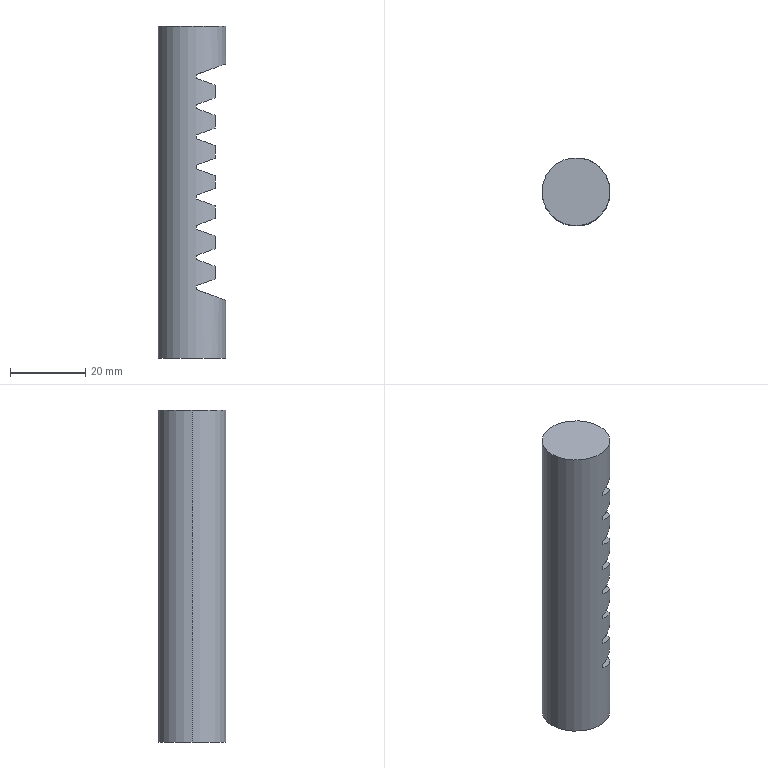Part | SolidWorks | features ICE 2, Extrusion 1, LPattern 1 | 1 solid | 35 faces | box 18 x 18 x 88 mm | volume 19025 mm3 | plane 33 | cylinder 2 | commonest cylinder face diameters 18 x2
STEP:
#1=CARTESIAN_POINT('',(9.,0.,44.));
#2=VERTEX_POINT('',#1);
#3=CARTESIAN_POINT('',(-9.,0.,44.));
#4=VERTEX_POINT('',#3);
#5=CARTESIAN_POINT('',(0.,0.,44.));
#6=DIRECTION('',(0.,0.,1.));
#7=DIRECTION('',(1.,0.,0.));
#8=AXIS2_PLACEMENT_3D('',#5,#6,#7);
#9=CIRCLE('',#8,9.);
#10=EDGE_CURVE('',#2,#4,#9,.T.);
#11=ORIENTED_EDGE('',*,*,#10,.F.);
#12=CARTESIAN_POINT('',(9.,0.,34.));
#13=VERTEX_POINT('',#12);
#14=CARTESIAN_POINT('',(9.,0.,44.));
#15=DIRECTION('',(0.,0.,-1.));
#16=VECTOR('',#15,1000.);
#17=LINE('',#14,#16);
#18=EDGE_CURVE('',#2,#13,#17,.T.);
#19=ORIENTED_EDGE('',*,*,#18,.T.);
#20=CARTESIAN_POINT('',(1.125,8.929,31.134));
#21=VERTEX_POINT('',#20);
#22=CARTESIAN_POINT('',(9.,0.,34.));
#23=CARTESIAN_POINT('',(9.,4.762,34.));
#24=CARTESIAN_POINT('',(5.85,8.334,32.853));
#25=CARTESIAN_POINT('',(1.125,8.929,31.134));
#26=(BOUNDED_CURVE()B_SPLINE_CURVE(3,(#22,#23,#24,#25),.UNSPECIFIED.,.F.,.F.)B_SPLINE_CURVE_WITH_KNOTS((4,4),(3.142,4.587),.UNSPECIFIED.)CURVE()GEOMETRIC_REPRESENTATION_ITEM()RATIONAL_B_SPLINE_CURVE((1.,0.8333,0.8333,1.))REPRESENTATION_ITEM(''));
#27=EDGE_CURVE('',#13,#21,#26,.T.);
#28=ORIENTED_EDGE('',*,*,#27,.T.);
#29=CARTESIAN_POINT('',(1.125,8.929,30.144));
#30=VERTEX_POINT('',#29);
#31=CARTESIAN_POINT('',(1.125,8.929,44.));
#32=DIRECTION('',(0.,0.,-1.));
#33=VECTOR('',#32,1000.);
#34=LINE('',#31,#33);
#35=EDGE_CURVE('',#21,#30,#34,.T.);
#36=ORIENTED_EDGE('',*,*,#35,.T.);
#37=CARTESIAN_POINT('',(6.142,6.579,28.318));
#38=VERTEX_POINT('',#37);
#39=CARTESIAN_POINT('',(1.125,8.929,30.144));
#40=CARTESIAN_POINT('',(3.019,8.691,29.454));
#41=CARTESIAN_POINT('',(4.747,7.881,28.825));
#42=CARTESIAN_POINT('',(6.142,6.579,28.318));
#43=(BOUNDED_CURVE()B_SPLINE_CURVE(3,(#39,#40,#41,#42),.UNSPECIFIED.,.F.,.F.)B_SPLINE_CURVE_WITH_KNOTS((4,4),(4.838,5.463),.UNSPECIFIED.)CURVE()GEOMETRIC_REPRESENTATION_ITEM()RATIONAL_B_SPLINE_CURVE((1.,0.9676,0.9676,1.))REPRESENTATION_ITEM(''));
#44=EDGE_CURVE('',#30,#38,#43,.T.);
#45=ORIENTED_EDGE('',*,*,#44,.T.);
#46=CARTESIAN_POINT('',(6.142,6.579,24.96));
#47=VERTEX_POINT('',#46);
#48=CARTESIAN_POINT('',(6.142,6.579,44.));
#49=DIRECTION('',(0.,0.,-1.));
#50=VECTOR('',#49,1000.);
#51=LINE('',#48,#50);
#52=EDGE_CURVE('',#38,#47,#51,.T.);
#53=ORIENTED_EDGE('',*,*,#52,.T.);
#54=CARTESIAN_POINT('',(1.125,8.929,23.134));
#55=VERTEX_POINT('',#54);
#56=CARTESIAN_POINT('',(6.142,6.579,24.96));
#57=CARTESIAN_POINT('',(4.747,7.881,24.452));
#58=CARTESIAN_POINT('',(3.019,8.691,23.823));
#59=CARTESIAN_POINT('',(1.125,8.929,23.134));
#60=(BOUNDED_CURVE()B_SPLINE_CURVE(3,(#56,#57,#58,#59),.UNSPECIFIED.,.F.,.F.)B_SPLINE_CURVE_WITH_KNOTS((4,4),(3.961,4.587),.UNSPECIFIED.)CURVE()GEOMETRIC_REPRESENTATION_ITEM()RATIONAL_B_SPLINE_CURVE((1.,0.9676,0.9676,1.))REPRESENTATION_ITEM(''));
#61=EDGE_CURVE('',#47,#55,#60,.T.);
#62=ORIENTED_EDGE('',*,*,#61,.T.);
#63=CARTESIAN_POINT('',(1.125,8.929,22.144));
#64=VERTEX_POINT('',#63);
#65=CARTESIAN_POINT('',(1.125,8.929,44.));
#66=DIRECTION('',(0.,0.,-1.));
#67=VECTOR('',#66,1000.);
#68=LINE('',#65,#67);
#69=EDGE_CURVE('',#55,#64,#68,.T.);
#70=ORIENTED_EDGE('',*,*,#69,.T.);
#71=CARTESIAN_POINT('',(6.142,6.579,20.318));
#72=VERTEX_POINT('',#71);
#73=CARTESIAN_POINT('',(1.125,8.929,22.144));
#74=CARTESIAN_POINT('',(3.019,8.691,21.454));
#75=CARTESIAN_POINT('',(4.747,7.881,20.825));
#76=CARTESIAN_POINT('',(6.142,6.579,20.318));
#77=(BOUNDED_CURVE()B_SPLINE_CURVE(3,(#73,#74,#75,#76),.UNSPECIFIED.,.F.,.T.)B_SPLINE_CURVE_WITH_KNOTS((4,4),(4.838,5.463),.UNSPECIFIED.)CURVE()GEOMETRIC_REPRESENTATION_ITEM()RATIONAL_B_SPLINE_CURVE((1.,0.9676,0.9676,1.))REPRESENTATION_ITEM(''));
#78=EDGE_CURVE('',#64,#72,#77,.T.);
#79=ORIENTED_EDGE('',*,*,#78,.T.);
#80=CARTESIAN_POINT('',(6.142,6.579,16.96));
#81=VERTEX_POINT('',#80);
#82=CARTESIAN_POINT('',(6.142,6.579,44.));
#83=DIRECTION('',(0.,0.,-1.));
#84=VECTOR('',#83,1000.);
#85=LINE('',#82,#84);
#86=EDGE_CURVE('',#72,#81,#85,.T.);
#87=ORIENTED_EDGE('',*,*,#86,.T.);
#88=CARTESIAN_POINT('',(1.125,8.929,15.134));
#89=VERTEX_POINT('',#88);
#90=CARTESIAN_POINT('',(6.142,6.579,16.96));
#91=CARTESIAN_POINT('',(4.747,7.881,16.452));
#92=CARTESIAN_POINT('',(3.019,8.691,15.823));
#93=CARTESIAN_POINT('',(1.125,8.929,15.134));
#94=(BOUNDED_CURVE()B_SPLINE_CURVE(3,(#90,#91,#92,#93),.UNSPECIFIED.,.F.,.F.)B_SPLINE_CURVE_WITH_KNOTS((4,4),(3.961,4.587),.UNSPECIFIED.)CURVE()GEOMETRIC_REPRESENTATION_ITEM()RATIONAL_B_SPLINE_CURVE((1.,0.9676,0.9676,1.))REPRESENTATION_ITEM(''));
#95=EDGE_CURVE('',#81,#89,#94,.T.);
#96=ORIENTED_EDGE('',*,*,#95,.T.);
#97=CARTESIAN_POINT('',(1.125,8.929,14.144));
#98=VERTEX_POINT('',#97);
#99=CARTESIAN_POINT('',(1.125,8.929,44.));
#100=DIRECTION('',(0.,0.,-1.));
#101=VECTOR('',#100,1000.);
#102=LINE('',#99,#101);
#103=EDGE_CURVE('',#89,#98,#102,.T.);
#104=ORIENTED_EDGE('',*,*,#103,.T.);
#105=CARTESIAN_POINT('',(6.142,6.579,12.318));
#106=VERTEX_POINT('',#105);
#107=CARTESIAN_POINT('',(1.125,8.929,14.144));
#108=CARTESIAN_POINT('',(3.019,8.691,13.454));
#109=CARTESIAN_POINT('',(4.747,7.881,12.825));
#110=CARTESIAN_POINT('',(6.142,6.579,12.318));
#111=(BOUNDED_CURVE()B_SPLINE_CURVE(3,(#107,#108,#109,#110),.UNSPECIFIED.,.F.,.F.)B_SPLINE_CURVE_WITH_KNOTS((4,4),(4.838,5.463),.UNSPECIFIED.)CURVE()GEOMETRIC_REPRESENTATION_ITEM()RATIONAL_B_SPLINE_CURVE((1.,0.9676,0.9676,1.))REPRESENTATION_ITEM(''));
#112=EDGE_CURVE('',#98,#106,#111,.T.);
#113=ORIENTED_EDGE('',*,*,#112,.T.);
#114=CARTESIAN_POINT('',(6.142,6.579,8.96));
#115=VERTEX_POINT('',#114);
#116=CARTESIAN_POINT('',(6.142,6.579,44.));
#117=DIRECTION('',(0.,0.,-1.));
#118=VECTOR('',#117,1000.);
#119=LINE('',#116,#118);
#120=EDGE_CURVE('',#106,#115,#119,.T.);
#121=ORIENTED_EDGE('',*,*,#120,.T.);
#122=CARTESIAN_POINT('',(1.125,8.929,7.134));
#123=VERTEX_POINT('',#122);
#124=CARTESIAN_POINT('',(6.142,6.579,8.96));
#125=CARTESIAN_POINT('',(4.747,7.881,8.452));
#126=CARTESIAN_POINT('',(3.019,8.691,7.823));
#127=CARTESIAN_POINT('',(1.125,8.929,7.134));
#128=(BOUNDED_CURVE()B_SPLINE_CURVE(3,(#124,#125,#126,#127),.UNSPECIFIED.,.F.,.F.)B_SPLINE_CURVE_WITH_KNOTS((4,4),(3.961,4.587),.UNSPECIFIED.)CURVE()GEOMETRIC_REPRESENTATION_ITEM()RATIONAL_B_SPLINE_CURVE((1.,0.9676,0.9676,1.))REPRESENTATION_ITEM(''));
#129=EDGE_CURVE('',#115,#123,#128,.T.);
#130=ORIENTED_EDGE('',*,*,#129,.T.);
#131=CARTESIAN_POINT('',(1.125,8.929,6.144));
#132=VERTEX_POINT('',#131);
#133=CARTESIAN_POINT('',(1.125,8.929,44.));
#134=DIRECTION('',(0.,0.,-1.));
#135=VECTOR('',#134,1000.);
#136=LINE('',#133,#135);
#137=EDGE_CURVE('',#123,#132,#136,.T.);
#138=ORIENTED_EDGE('',*,*,#137,.T.);
#139=CARTESIAN_POINT('',(6.142,6.579,4.318));
#140=VERTEX_POINT('',#139);
#141=CARTESIAN_POINT('',(1.125,8.929,6.144));
#142=CARTESIAN_POINT('',(3.019,8.691,5.454));
#143=CARTESIAN_POINT('',(4.747,7.881,4.825));
#144=CARTESIAN_POINT('',(6.142,6.579,4.318));
#145=(BOUNDED_CURVE()B_SPLINE_CURVE(3,(#141,#142,#143,#144),.UNSPECIFIED.,.F.,.F.)B_SPLINE_CURVE_WITH_KNOTS((4,4),(4.838,5.463),.UNSPECIFIED.)CURVE()GEOMETRIC_REPRESENTATION_ITEM()RATIONAL_B_SPLINE_CURVE((1.,0.9676,0.9676,1.))REPRESENTATION_ITEM(''));
#146=EDGE_CURVE('',#132,#140,#145,.T.);
#147=ORIENTED_EDGE('',*,*,#146,.T.);
#148=CARTESIAN_POINT('',(6.142,6.579,0.9597));
#149=VERTEX_POINT('',#148);
#150=CARTESIAN_POINT('',(6.142,6.579,44.));
#151=DIRECTION('',(0.,0.,-1.));
#152=VECTOR('',#151,1000.);
#153=LINE('',#150,#152);
#154=EDGE_CURVE('',#140,#149,#153,.T.);
#155=ORIENTED_EDGE('',*,*,#154,.T.);
#156=CARTESIAN_POINT('',(1.125,8.929,-0.8663));
#157=VERTEX_POINT('',#156);
#158=CARTESIAN_POINT('',(6.142,6.579,0.9597));
#159=CARTESIAN_POINT('',(4.747,7.881,0.452));
#160=CARTESIAN_POINT('',(3.019,8.691,-0.177));
#161=CARTESIAN_POINT('',(1.125,8.929,-0.8663));
#162=(BOUNDED_CURVE()B_SPLINE_CURVE(3,(#158,#159,#160,#161),.UNSPECIFIED.,.F.,.T.)B_SPLINE_CURVE_WITH_KNOTS((4,4),(3.961,4.587),.UNSPECIFIED.)CURVE()GEOMETRIC_REPRESENTATION_ITEM()RATIONAL_B_SPLINE_CURVE((1.,0.9676,0.9676,1.))REPRESENTATION_ITEM(''));
#163=EDGE_CURVE('',#149,#157,#162,.T.);
#164=ORIENTED_EDGE('',*,*,#163,.T.);
#165=CARTESIAN_POINT('',(1.125,8.929,-1.856));
#166=VERTEX_POINT('',#165);
#167=CARTESIAN_POINT('',(1.125,8.929,44.));
#168=DIRECTION('',(0.,0.,-1.));
#169=VECTOR('',#168,1000.);
#170=LINE('',#167,#169);
#171=EDGE_CURVE('',#157,#166,#170,.T.);
#172=ORIENTED_EDGE('',*,*,#171,.T.);
#173=CARTESIAN_POINT('',(6.142,6.579,-3.682));
#174=VERTEX_POINT('',#173);
#175=CARTESIAN_POINT('',(1.125,8.929,-1.856));
#176=CARTESIAN_POINT('',(3.019,8.691,-2.546));
#177=CARTESIAN_POINT('',(4.747,7.881,-3.175));
#178=CARTESIAN_POINT('',(6.142,6.579,-3.682));
#179=(BOUNDED_CURVE()B_SPLINE_CURVE(3,(#175,#176,#177,#178),.UNSPECIFIED.,.F.,.F.)B_SPLINE_CURVE_WITH_KNOTS((4,4),(4.838,5.463),.UNSPECIFIED.)CURVE()GEOMETRIC_REPRESENTATION_ITEM()RATIONAL_B_SPLINE_CURVE((1.,0.9676,0.9676,1.))REPRESENTATION_ITEM(''));
#180=EDGE_CURVE('',#166,#174,#179,.T.);
#181=ORIENTED_EDGE('',*,*,#180,.T.);
#182=CARTESIAN_POINT('',(6.142,6.579,-7.04));
#183=VERTEX_POINT('',#182);
#184=CARTESIAN_POINT('',(6.142,6.579,44.));
#185=DIRECTION('',(0.,0.,-1.));
#186=VECTOR('',#185,1000.);
#187=LINE('',#184,#186);
#188=EDGE_CURVE('',#174,#183,#187,.T.);
#189=ORIENTED_EDGE('',*,*,#188,.T.);
#190=CARTESIAN_POINT('',(1.125,8.929,-8.866));
#191=VERTEX_POINT('',#190);
#192=CARTESIAN_POINT('',(6.142,6.579,-7.04));
#193=CARTESIAN_POINT('',(4.747,7.881,-7.548));
#194=CARTESIAN_POINT('',(3.019,8.691,-8.177));
#195=CARTESIAN_POINT('',(1.125,8.929,-8.866));
#196=(BOUNDED_CURVE()B_SPLINE_CURVE(3,(#192,#193,#194,#195),.UNSPECIFIED.,.F.,.F.)B_SPLINE_CURVE_WITH_KNOTS((4,4),(3.961,4.587),.UNSPECIFIED.)CURVE()GEOMETRIC_REPRESENTATION_ITEM()RATIONAL_B_SPLINE_CURVE((1.,0.9676,0.9676,1.))REPRESENTATION_ITEM(''));
#197=EDGE_CURVE('',#183,#191,#196,.T.);
#198=ORIENTED_EDGE('',*,*,#197,.T.);
#199=CARTESIAN_POINT('',(1.125,8.929,-9.856));
#200=VERTEX_POINT('',#199);
#201=CARTESIAN_POINT('',(1.125,8.929,44.));
#202=DIRECTION('',(0.,0.,-1.));
#203=VECTOR('',#202,1000.);
#204=LINE('',#201,#203);
#205=EDGE_CURVE('',#191,#200,#204,.T.);
#206=ORIENTED_EDGE('',*,*,#205,.T.);
#207=CARTESIAN_POINT('',(6.142,6.579,-11.682));
#208=VERTEX_POINT('',#207);
#209=CARTESIAN_POINT('',(1.125,8.929,-9.856));
#210=CARTESIAN_POINT('',(3.019,8.691,-10.546));
#211=CARTESIAN_POINT('',(4.747,7.881,-11.175));
#212=CARTESIAN_POINT('',(6.142,6.579,-11.682));
#213=(BOUNDED_CURVE()B_SPLINE_CURVE(3,(#209,#210,#211,#212),.UNSPECIFIED.,.F.,.F.)B_SPLINE_CURVE_WITH_KNOTS((4,4),(4.838,5.463),.UNSPECIFIED.)CURVE()GEOMETRIC_REPRESENTATION_ITEM()RATIONAL_B_SPLINE_CURVE((1.,0.9676,0.9676,1.))REPRESENTATION_ITEM(''));
#214=EDGE_CURVE('',#200,#208,#213,.T.);
#215=ORIENTED_EDGE('',*,*,#214,.T.);
#216=CARTESIAN_POINT('',(6.142,6.579,-15.04));
#217=VERTEX_POINT('',#216);
#218=CARTESIAN_POINT('',(6.142,6.579,44.));
#219=DIRECTION('',(0.,0.,-1.));
#220=VECTOR('',#219,1000.);
#221=LINE('',#218,#220);
#222=EDGE_CURVE('',#208,#217,#221,.T.);
#223=ORIENTED_EDGE('',*,*,#222,.T.);
#224=CARTESIAN_POINT('',(1.125,8.929,-16.866));
#225=VERTEX_POINT('',#224);
#226=CARTESIAN_POINT('',(6.142,6.579,-15.04));
#227=CARTESIAN_POINT('',(4.747,7.881,-15.548));
#228=CARTESIAN_POINT('',(3.019,8.691,-16.177));
#229=CARTESIAN_POINT('',(1.125,8.929,-16.866));
#230=(BOUNDED_CURVE()B_SPLINE_CURVE(3,(#226,#227,#228,#229),.UNSPECIFIED.,.F.,.T.)B_SPLINE_CURVE_WITH_KNOTS((4,4),(3.961,4.587),.UNSPECIFIED.)CURVE()GEOMETRIC_REPRESENTATION_ITEM()RATIONAL_B_SPLINE_CURVE((1.,0.9676,0.9676,1.))REPRESENTATION_ITEM(''));
#231=EDGE_CURVE('',#217,#225,#230,.T.);
#232=ORIENTED_EDGE('',*,*,#231,.T.);
#233=CARTESIAN_POINT('',(1.125,8.929,-17.856));
#234=VERTEX_POINT('',#233);
#235=CARTESIAN_POINT('',(1.125,8.929,44.));
#236=DIRECTION('',(0.,0.,-1.));
#237=VECTOR('',#236,1000.);
#238=LINE('',#235,#237);
#239=EDGE_CURVE('',#225,#234,#238,.T.);
#240=ORIENTED_EDGE('',*,*,#239,.T.);
#241=CARTESIAN_POINT('',(6.142,6.579,-19.682));
#242=VERTEX_POINT('',#241);
#243=CARTESIAN_POINT('',(1.125,8.929,-17.856));
#244=CARTESIAN_POINT('',(3.019,8.691,-18.546));
#245=CARTESIAN_POINT('',(4.747,7.881,-19.175));
#246=CARTESIAN_POINT('',(6.142,6.579,-19.682));
#247=(BOUNDED_CURVE()B_SPLINE_CURVE(3,(#243,#244,#245,#246),.UNSPECIFIED.,.F.,.T.)B_SPLINE_CURVE_WITH_KNOTS((4,4),(4.838,5.463),.UNSPECIFIED.)CURVE()GEOMETRIC_REPRESENTATION_ITEM()RATIONAL_B_SPLINE_CURVE((1.,0.9676,0.9676,1.))REPRESENTATION_ITEM(''));
#248=EDGE_CURVE('',#234,#242,#247,.T.);
#249=ORIENTED_EDGE('',*,*,#248,.T.);
#250=CARTESIAN_POINT('',(6.142,6.579,-23.04));
#251=VERTEX_POINT('',#250);
#252=CARTESIAN_POINT('',(6.142,6.579,44.));
#253=DIRECTION('',(0.,0.,-1.));
#254=VECTOR('',#253,1000.);
#255=LINE('',#252,#254);
#256=EDGE_CURVE('',#242,#251,#255,.T.);
#257=ORIENTED_EDGE('',*,*,#256,.T.);
#258=CARTESIAN_POINT('',(1.125,8.929,-24.866));
#259=VERTEX_POINT('',#258);
#260=CARTESIAN_POINT('',(6.142,6.579,-23.04));
#261=CARTESIAN_POINT('',(4.747,7.881,-23.548));
#262=CARTESIAN_POINT('',(3.019,8.691,-24.177));
#263=CARTESIAN_POINT('',(1.125,8.929,-24.866));
#264=(BOUNDED_CURVE()B_SPLINE_CURVE(3,(#260,#261,#262,#263),.UNSPECIFIED.,.F.,.F.)B_SPLINE_CURVE_WITH_KNOTS((4,4),(3.961,4.587),.UNSPECIFIED.)CURVE()GEOMETRIC_REPRESENTATION_ITEM()RATIONAL_B_SPLINE_CURVE((1.,0.9676,0.9676,1.))REPRESENTATION_ITEM(''));
#265=EDGE_CURVE('',#251,#259,#264,.T.);
#266=ORIENTED_EDGE('',*,*,#265,.T.);
#267=CARTESIAN_POINT('',(1.125,8.929,-25.856));
#268=VERTEX_POINT('',#267);
#269=CARTESIAN_POINT('',(1.125,8.929,44.));
#270=DIRECTION('',(0.,0.,-1.));
#271=VECTOR('',#270,1000.);
#272=LINE('',#269,#271);
#273=EDGE_CURVE('',#259,#268,#272,.T.);
#274=ORIENTED_EDGE('',*,*,#273,.T.);
#275=CARTESIAN_POINT('',(9.,0.,-28.723));
#276=VERTEX_POINT('',#275);
#277=CARTESIAN_POINT('',(1.125,8.929,-25.856));
#278=CARTESIAN_POINT('',(5.85,8.334,-27.576));
#279=CARTESIAN_POINT('',(9.,4.762,-28.723));
#280=CARTESIAN_POINT('',(9.,0.,-28.723));
#281=(BOUNDED_CURVE()B_SPLINE_CURVE(3,(#277,#278,#279,#280),.UNSPECIFIED.,.F.,.T.)B_SPLINE_CURVE_WITH_KNOTS((4,4),(4.838,6.283),.UNSPECIFIED.)CURVE()GEOMETRIC_REPRESENTATION_ITEM()RATIONAL_B_SPLINE_CURVE((1.,0.8333,0.8333,1.))REPRESENTATION_ITEM(''));
#282=EDGE_CURVE('',#268,#276,#281,.T.);
#283=ORIENTED_EDGE('',*,*,#282,.T.);
#284=CARTESIAN_POINT('',(9.,0.,-44.));
#285=VERTEX_POINT('',#284);
#286=CARTESIAN_POINT('',(9.,0.,44.));
#287=DIRECTION('',(0.,0.,-1.));
#288=VECTOR('',#287,1000.);
#289=LINE('',#286,#288);
#290=EDGE_CURVE('',#276,#285,#289,.T.);
#291=ORIENTED_EDGE('',*,*,#290,.T.);
#292=CARTESIAN_POINT('',(-9.,0.,-44.));
#293=VERTEX_POINT('',#292);
#294=CARTESIAN_POINT('',(0.,0.,-44.));
#295=DIRECTION('',(0.,0.,1.));
#296=DIRECTION('',(1.,0.,0.));
#297=AXIS2_PLACEMENT_3D('',#294,#295,#296);
#298=CIRCLE('',#297,9.);
#299=EDGE_CURVE('',#285,#293,#298,.T.);
#300=ORIENTED_EDGE('',*,*,#299,.T.);
#301=CARTESIAN_POINT('',(-9.,0.,44.));
#302=DIRECTION('',(0.,0.,-1.));
#303=VECTOR('',#302,1000.);
#304=LINE('',#301,#303);
#305=EDGE_CURVE('',#4,#293,#304,.T.);
#306=ORIENTED_EDGE('',*,*,#305,.F.);
#307=EDGE_LOOP('',(#11,#19,#28,#36,#45,#53,#62,#70,#79,#87,#96,#104,#113,#121,#130,#138,#147,#155,#164,#172,#181,#189,#198,#206,#215,#223,#232,#240,#249,#257,#266,#274,#283,#291,#300,#306));
#308=FACE_OUTER_BOUND('',#307,.T.);
#309=CARTESIAN_POINT('',(0.,0.,44.));
#310=DIRECTION('',(0.,0.,-1.));
#311=DIRECTION('',(-1.,0.,0.));
#312=AXIS2_PLACEMENT_3D('',#309,#310,#311);
#313=CYLINDRICAL_SURFACE('',#312,9.);
#314=ADVANCED_FACE('',(#308),#313,.T.);
#315=ORIENTED_EDGE('',*,*,#18,.F.);
#316=CARTESIAN_POINT('',(0.,0.,44.));
#317=DIRECTION('',(0.,0.,1.));
#318=DIRECTION('',(1.,0.,0.));
#319=AXIS2_PLACEMENT_3D('',#316,#317,#318);
#320=CIRCLE('',#319,9.);
#321=EDGE_CURVE('',#4,#2,#320,.T.);
#322=ORIENTED_EDGE('',*,*,#321,.F.);
#323=ORIENTED_EDGE('',*,*,#305,.T.);
#324=CARTESIAN_POINT('',(0.,0.,-44.));
#325=DIRECTION('',(0.,0.,1.));
#326=DIRECTION('',(1.,0.,0.));
#327=AXIS2_PLACEMENT_3D('',#324,#325,#326);
#328=CIRCLE('',#327,9.);
#329=EDGE_CURVE('',#293,#285,#328,.T.);
#330=ORIENTED_EDGE('',*,*,#329,.T.);
#331=ORIENTED_EDGE('',*,*,#290,.F.);
#332=CARTESIAN_POINT('',(1.125,-8.929,-25.856));
#333=VERTEX_POINT('',#332);
#334=CARTESIAN_POINT('',(9.,0.,-28.723));
#335=CARTESIAN_POINT('',(9.,-4.762,-28.723));
#336=CARTESIAN_POINT('',(5.85,-8.334,-27.576));
#337=CARTESIAN_POINT('',(1.125,-8.929,-25.856));
#338=(BOUNDED_CURVE()B_SPLINE_CURVE(3,(#334,#335,#336,#337),.UNSPECIFIED.,.F.,.F.)B_SPLINE_CURVE_WITH_KNOTS((4,4),(0.,1.445),.UNSPECIFIED.)CURVE()GEOMETRIC_REPRESENTATION_ITEM()RATIONAL_B_SPLINE_CURVE((1.,0.8333,0.8333,1.))REPRESENTATION_ITEM(''));
#339=EDGE_CURVE('',#276,#333,#338,.T.);
#340=ORIENTED_EDGE('',*,*,#339,.T.);
#341=CARTESIAN_POINT('',(1.125,-8.929,-24.866));
#342=VERTEX_POINT('',#341);
#343=CARTESIAN_POINT('',(1.125,-8.929,44.));
#344=DIRECTION('',(0.,0.,1.));
#345=VECTOR('',#344,1000.);
#346=LINE('',#343,#345);
#347=EDGE_CURVE('',#333,#342,#346,.T.);
#348=ORIENTED_EDGE('',*,*,#347,.T.);
#349=CARTESIAN_POINT('',(6.142,-6.579,-23.04));
#350=VERTEX_POINT('',#349);
#351=CARTESIAN_POINT('',(1.125,-8.929,-24.866));
#352=CARTESIAN_POINT('',(3.019,-8.691,-24.177));
#353=CARTESIAN_POINT('',(4.747,-7.881,-23.548));
#354=CARTESIAN_POINT('',(6.142,-6.579,-23.04));
#355=(BOUNDED_CURVE()B_SPLINE_CURVE(3,(#351,#352,#353,#354),.UNSPECIFIED.,.F.,.T.)B_SPLINE_CURVE_WITH_KNOTS((4,4),(1.696,2.322),.UNSPECIFIED.)CURVE()GEOMETRIC_REPRESENTATION_ITEM()RATIONAL_B_SPLINE_CURVE((1.,0.9676,0.9676,1.))REPRESENTATION_ITEM(''));
#356=EDGE_CURVE('',#342,#350,#355,.T.);
#357=ORIENTED_EDGE('',*,*,#356,.T.);
#358=CARTESIAN_POINT('',(6.142,-6.579,-19.682));
#359=VERTEX_POINT('',#358);
#360=CARTESIAN_POINT('',(6.142,-6.579,44.));
#361=DIRECTION('',(0.,0.,1.));
#362=VECTOR('',#361,1000.);
#363=LINE('',#360,#362);
#364=EDGE_CURVE('',#350,#359,#363,.T.);
#365=ORIENTED_EDGE('',*,*,#364,.T.);
#366=CARTESIAN_POINT('',(1.125,-8.929,-17.856));
#367=VERTEX_POINT('',#366);
#368=CARTESIAN_POINT('',(6.142,-6.579,-19.682));
#369=CARTESIAN_POINT('',(4.747,-7.881,-19.175));
#370=CARTESIAN_POINT('',(3.019,-8.691,-18.546));
#371=CARTESIAN_POINT('',(1.125,-8.929,-17.856));
#372=(BOUNDED_CURVE()B_SPLINE_CURVE(3,(#368,#369,#370,#371),.UNSPECIFIED.,.F.,.T.)B_SPLINE_CURVE_WITH_KNOTS((4,4),(0.8197,1.445),.UNSPECIFIED.)CURVE()GEOMETRIC_REPRESENTATION_ITEM()RATIONAL_B_SPLINE_CURVE((1.,0.9676,0.9676,1.))REPRESENTATION_ITEM(''));
#373=EDGE_CURVE('',#359,#367,#372,.T.);
#374=ORIENTED_EDGE('',*,*,#373,.T.);
#375=CARTESIAN_POINT('',(1.125,-8.929,-16.866));
#376=VERTEX_POINT('',#375);
#377=CARTESIAN_POINT('',(1.125,-8.929,44.));
#378=DIRECTION('',(0.,0.,1.));
#379=VECTOR('',#378,1000.);
#380=LINE('',#377,#379);
#381=EDGE_CURVE('',#367,#376,#380,.T.);
#382=ORIENTED_EDGE('',*,*,#381,.T.);
#383=CARTESIAN_POINT('',(6.142,-6.579,-15.04));
#384=VERTEX_POINT('',#383);
#385=CARTESIAN_POINT('',(1.125,-8.929,-16.866));
#386=CARTESIAN_POINT('',(3.019,-8.691,-16.177));
#387=CARTESIAN_POINT('',(4.747,-7.881,-15.548));
#388=CARTESIAN_POINT('',(6.142,-6.579,-15.04));
#389=(BOUNDED_CURVE()B_SPLINE_CURVE(3,(#385,#386,#387,#388),.UNSPECIFIED.,.F.,.T.)B_SPLINE_CURVE_WITH_KNOTS((4,4),(1.696,2.322),.UNSPECIFIED.)CURVE()GEOMETRIC_REPRESENTATION_ITEM()RATIONAL_B_SPLINE_CURVE((1.,0.9676,0.9676,1.))REPRESENTATION_ITEM(''));
#390=EDGE_CURVE('',#376,#384,#389,.T.);
#391=ORIENTED_EDGE('',*,*,#390,.T.);
#392=CARTESIAN_POINT('',(6.142,-6.579,-11.682));
#393=VERTEX_POINT('',#392);
#394=CARTESIAN_POINT('',(6.142,-6.579,44.));
#395=DIRECTION('',(0.,0.,1.));
#396=VECTOR('',#395,1000.);
#397=LINE('',#394,#396);
#398=EDGE_CURVE('',#384,#393,#397,.T.);
#399=ORIENTED_EDGE('',*,*,#398,.T.);
#400=CARTESIAN_POINT('',(1.125,-8.929,-9.856));
#401=VERTEX_POINT('',#400);
#402=CARTESIAN_POINT('',(6.142,-6.579,-11.682));
#403=CARTESIAN_POINT('',(4.747,-7.881,-11.175));
#404=CARTESIAN_POINT('',(3.019,-8.691,-10.546));
#405=CARTESIAN_POINT('',(1.125,-8.929,-9.856));
#406=(BOUNDED_CURVE()B_SPLINE_CURVE(3,(#402,#403,#404,#405),.UNSPECIFIED.,.F.,.T.)B_SPLINE_CURVE_WITH_KNOTS((4,4),(0.8197,1.445),.UNSPECIFIED.)CURVE()GEOMETRIC_REPRESENTATION_ITEM()RATIONAL_B_SPLINE_CURVE((1.,0.9676,0.9676,1.))REPRESENTATION_ITEM(''));
#407=EDGE_CURVE('',#393,#401,#406,.T.);
#408=ORIENTED_EDGE('',*,*,#407,.T.);
#409=CARTESIAN_POINT('',(1.125,-8.929,-8.866));
#410=VERTEX_POINT('',#409);
#411=CARTESIAN_POINT('',(1.125,-8.929,44.));
#412=DIRECTION('',(0.,0.,1.));
#413=VECTOR('',#412,1000.);
#414=LINE('',#411,#413);
#415=EDGE_CURVE('',#401,#410,#414,.T.);
#416=ORIENTED_EDGE('',*,*,#415,.T.);
#417=CARTESIAN_POINT('',(6.142,-6.579,-7.04));
#418=VERTEX_POINT('',#417);
#419=CARTESIAN_POINT('',(1.125,-8.929,-8.866));
#420=CARTESIAN_POINT('',(3.019,-8.691,-8.177));
#421=CARTESIAN_POINT('',(4.747,-7.881,-7.548));
#422=CARTESIAN_POINT('',(6.142,-6.579,-7.04));
#423=(BOUNDED_CURVE()B_SPLINE_CURVE(3,(#419,#420,#421,#422),.UNSPECIFIED.,.F.,.F.)B_SPLINE_CURVE_WITH_KNOTS((4,4),(1.696,2.322),.UNSPECIFIED.)CURVE()GEOMETRIC_REPRESENTATION_ITEM()RATIONAL_B_SPLINE_CURVE((1.,0.9676,0.9676,1.))REPRESENTATION_ITEM(''));
#424=EDGE_CURVE('',#410,#418,#423,.T.);
#425=ORIENTED_EDGE('',*,*,#424,.T.);
#426=CARTESIAN_POINT('',(6.142,-6.579,-3.682));
#427=VERTEX_POINT('',#426);
#428=CARTESIAN_POINT('',(6.142,-6.579,44.));
#429=DIRECTION('',(0.,0.,1.));
#430=VECTOR('',#429,1000.);
#431=LINE('',#428,#430);
#432=EDGE_CURVE('',#418,#427,#431,.T.);
#433=ORIENTED_EDGE('',*,*,#432,.T.);
#434=CARTESIAN_POINT('',(1.125,-8.929,-1.856));
#435=VERTEX_POINT('',#434);
#436=CARTESIAN_POINT('',(6.142,-6.579,-3.682));
#437=CARTESIAN_POINT('',(4.747,-7.881,-3.175));
#438=CARTESIAN_POINT('',(3.019,-8.691,-2.546));
#439=CARTESIAN_POINT('',(1.125,-8.929,-1.856));
#440=(BOUNDED_CURVE()B_SPLINE_CURVE(3,(#436,#437,#438,#439),.UNSPECIFIED.,.F.,.T.)B_SPLINE_CURVE_WITH_KNOTS((4,4),(0.8197,1.445),.UNSPECIFIED.)CURVE()GEOMETRIC_REPRESENTATION_ITEM()RATIONAL_B_SPLINE_CURVE((1.,0.9676,0.9676,1.))REPRESENTATION_ITEM(''));
#441=EDGE_CURVE('',#427,#435,#440,.T.);
#442=ORIENTED_EDGE('',*,*,#441,.T.);
#443=CARTESIAN_POINT('',(1.125,-8.929,-0.8663));
#444=VERTEX_POINT('',#443);
#445=CARTESIAN_POINT('',(1.125,-8.929,44.));
#446=DIRECTION('',(0.,0.,1.));
#447=VECTOR('',#446,1000.);
#448=LINE('',#445,#447);
#449=EDGE_CURVE('',#435,#444,#448,.T.);
#450=ORIENTED_EDGE('',*,*,#449,.T.);
#451=CARTESIAN_POINT('',(6.142,-6.579,0.9597));
#452=VERTEX_POINT('',#451);
#453=CARTESIAN_POINT('',(1.125,-8.929,-0.8663));
#454=CARTESIAN_POINT('',(3.019,-8.691,-0.177));
#455=CARTESIAN_POINT('',(4.747,-7.881,0.452));
#456=CARTESIAN_POINT('',(6.142,-6.579,0.9597));
#457=(BOUNDED_CURVE()B_SPLINE_CURVE(3,(#453,#454,#455,#456),.UNSPECIFIED.,.F.,.T.)B_SPLINE_CURVE_WITH_KNOTS((4,4),(1.696,2.322),.UNSPECIFIED.)CURVE()GEOMETRIC_REPRESENTATION_ITEM()RATIONAL_B_SPLINE_CURVE((1.,0.9676,0.9676,1.))REPRESENTATION_ITEM(''));
#458=EDGE_CURVE('',#444,#452,#457,.T.);
#459=ORIENTED_EDGE('',*,*,#458,.T.);
#460=CARTESIAN_POINT('',(6.142,-6.579,4.318));
#461=VERTEX_POINT('',#460);
#462=CARTESIAN_POINT('',(6.142,-6.579,44.));
#463=DIRECTION('',(0.,0.,1.));
#464=VECTOR('',#463,1000.);
#465=LINE('',#462,#464);
#466=EDGE_CURVE('',#452,#461,#465,.T.);
#467=ORIENTED_EDGE('',*,*,#466,.T.);
#468=CARTESIAN_POINT('',(1.125,-8.929,6.144));
#469=VERTEX_POINT('',#468);
#470=CARTESIAN_POINT('',(6.142,-6.579,4.318));
#471=CARTESIAN_POINT('',(4.747,-7.881,4.825));
#472=CARTESIAN_POINT('',(3.019,-8.691,5.454));
#473=CARTESIAN_POINT('',(1.125,-8.929,6.144));
#474=(BOUNDED_CURVE()B_SPLINE_CURVE(3,(#470,#471,#472,#473),.UNSPECIFIED.,.F.,.F.)B_SPLINE_CURVE_WITH_KNOTS((4,4),(0.8197,1.445),.UNSPECIFIED.)CURVE()GEOMETRIC_REPRESENTATION_ITEM()RATIONAL_B_SPLINE_CURVE((1.,0.9676,0.9676,1.))REPRESENTATION_ITEM(''));
#475=EDGE_CURVE('',#461,#469,#474,.T.);
#476=ORIENTED_EDGE('',*,*,#475,.T.);
#477=CARTESIAN_POINT('',(1.125,-8.929,7.134));
#478=VERTEX_POINT('',#477);
#479=CARTESIAN_POINT('',(1.125,-8.929,44.));
#480=DIRECTION('',(0.,0.,1.));
#481=VECTOR('',#480,1000.);
#482=LINE('',#479,#481);
#483=EDGE_CURVE('',#469,#478,#482,.T.);
#484=ORIENTED_EDGE('',*,*,#483,.T.);
#485=CARTESIAN_POINT('',(6.142,-6.579,8.96));
#486=VERTEX_POINT('',#485);
#487=CARTESIAN_POINT('',(1.125,-8.929,7.134));
#488=CARTESIAN_POINT('',(3.019,-8.691,7.823));
#489=CARTESIAN_POINT('',(4.747,-7.881,8.452));
#490=CARTESIAN_POINT('',(6.142,-6.579,8.96));
#491=(BOUNDED_CURVE()B_SPLINE_CURVE(3,(#487,#488,#489,#490),.UNSPECIFIED.,.F.,.T.)B_SPLINE_CURVE_WITH_KNOTS((4,4),(1.696,2.322),.UNSPECIFIED.)CURVE()GEOMETRIC_REPRESENTATION_ITEM()RATIONAL_B_SPLINE_CURVE((1.,0.9676,0.9676,1.))REPRESENTATION_ITEM(''));
#492=EDGE_CURVE('',#478,#486,#491,.T.);
#493=ORIENTED_EDGE('',*,*,#492,.T.);
#494=CARTESIAN_POINT('',(6.142,-6.579,12.318));
#495=VERTEX_POINT('',#494);
#496=CARTESIAN_POINT('',(6.142,-6.579,44.));
#497=DIRECTION('',(0.,0.,1.));
#498=VECTOR('',#497,1000.);
#499=LINE('',#496,#498);
#500=EDGE_CURVE('',#486,#495,#499,.T.);
#501=ORIENTED_EDGE('',*,*,#500,.T.);
#502=CARTESIAN_POINT('',(1.125,-8.929,14.144));
#503=VERTEX_POINT('',#502);
#504=CARTESIAN_POINT('',(6.142,-6.579,12.318));
#505=CARTESIAN_POINT('',(4.747,-7.881,12.825));
#506=CARTESIAN_POINT('',(3.019,-8.691,13.454));
#507=CARTESIAN_POINT('',(1.125,-8.929,14.144));
#508=(BOUNDED_CURVE()B_SPLINE_CURVE(3,(#504,#505,#506,#507),.UNSPECIFIED.,.F.,.T.)B_SPLINE_CURVE_WITH_KNOTS((4,4),(0.8197,1.445),.UNSPECIFIED.)CURVE()GEOMETRIC_REPRESENTATION_ITEM()RATIONAL_B_SPLINE_CURVE((1.,0.9676,0.9676,1.))REPRESENTATION_ITEM(''));
#509=EDGE_CURVE('',#495,#503,#508,.T.);
#510=ORIENTED_EDGE('',*,*,#509,.T.);
#511=CARTESIAN_POINT('',(1.125,-8.929,15.134));
#512=VERTEX_POINT('',#511);
#513=CARTESIAN_POINT('',(1.125,-8.929,44.));
#514=DIRECTION('',(0.,0.,1.));
#515=VECTOR('',#514,1000.);
#516=LINE('',#513,#515);
#517=EDGE_CURVE('',#503,#512,#516,.T.);
#518=ORIENTED_EDGE('',*,*,#517,.T.);
#519=CARTESIAN_POINT('',(6.142,-6.579,16.96));
#520=VERTEX_POINT('',#519);
#521=CARTESIAN_POINT('',(1.125,-8.929,15.134));
#522=CARTESIAN_POINT('',(3.019,-8.691,15.823));
#523=CARTESIAN_POINT('',(4.747,-7.881,16.452));
#524=CARTESIAN_POINT('',(6.142,-6.579,16.96));
#525=(BOUNDED_CURVE()B_SPLINE_CURVE(3,(#521,#522,#523,#524),.UNSPECIFIED.,.F.,.T.)B_SPLINE_CURVE_WITH_KNOTS((4,4),(1.696,2.322),.UNSPECIFIED.)CURVE()GEOMETRIC_REPRESENTATION_ITEM()RATIONAL_B_SPLINE_CURVE((1.,0.9676,0.9676,1.))REPRESENTATION_ITEM(''));
#526=EDGE_CURVE('',#512,#520,#525,.T.);
#527=ORIENTED_EDGE('',*,*,#526,.T.);
#528=CARTESIAN_POINT('',(6.142,-6.579,20.318));
#529=VERTEX_POINT('',#528);
#530=CARTESIAN_POINT('',(6.142,-6.579,44.));
#531=DIRECTION('',(0.,0.,1.));
#532=VECTOR('',#531,1000.);
#533=LINE('',#530,#532);
#534=EDGE_CURVE('',#520,#529,#533,.T.);
#535=ORIENTED_EDGE('',*,*,#534,.T.);
#536=CARTESIAN_POINT('',(1.125,-8.929,22.144));
#537=VERTEX_POINT('',#536);
#538=CARTESIAN_POINT('',(6.142,-6.579,20.318));
#539=CARTESIAN_POINT('',(4.747,-7.881,20.825));
#540=CARTESIAN_POINT('',(3.019,-8.691,21.454));
#541=CARTESIAN_POINT('',(1.125,-8.929,22.144));
#542=(BOUNDED_CURVE()B_SPLINE_CURVE(3,(#538,#539,#540,#541),.UNSPECIFIED.,.F.,.T.)B_SPLINE_CURVE_WITH_KNOTS((4,4),(0.8197,1.445),.UNSPECIFIED.)CURVE()GEOMETRIC_REPRESENTATION_ITEM()RATIONAL_B_SPLINE_CURVE((1.,0.9676,0.9676,1.))REPRESENTATION_ITEM(''));
#543=EDGE_CURVE('',#529,#537,#542,.T.);
#544=ORIENTED_EDGE('',*,*,#543,.T.);
#545=CARTESIAN_POINT('',(1.125,-8.929,23.134));
#546=VERTEX_POINT('',#545);
#547=CARTESIAN_POINT('',(1.125,-8.929,44.));
#548=DIRECTION('',(0.,0.,1.));
#549=VECTOR('',#548,1000.);
#550=LINE('',#547,#549);
#551=EDGE_CURVE('',#537,#546,#550,.T.);
#552=ORIENTED_EDGE('',*,*,#551,.T.);
#553=CARTESIAN_POINT('',(6.142,-6.579,24.96));
#554=VERTEX_POINT('',#553);
#555=CARTESIAN_POINT('',(1.125,-8.929,23.134));
#556=CARTESIAN_POINT('',(3.019,-8.691,23.823));
#557=CARTESIAN_POINT('',(4.747,-7.881,24.452));
#558=CARTESIAN_POINT('',(6.142,-6.579,24.96));
#559=(BOUNDED_CURVE()B_SPLINE_CURVE(3,(#555,#556,#557,#558),.UNSPECIFIED.,.F.,.T.)B_SPLINE_CURVE_WITH_KNOTS((4,4),(1.696,2.322),.UNSPECIFIED.)CURVE()GEOMETRIC_REPRESENTATION_ITEM()RATIONAL_B_SPLINE_CURVE((1.,0.9676,0.9676,1.))REPRESENTATION_ITEM(''));
#560=EDGE_CURVE('',#546,#554,#559,.T.);
#561=ORIENTED_EDGE('',*,*,#560,.T.);
#562=CARTESIAN_POINT('',(6.142,-6.579,28.318));
#563=VERTEX_POINT('',#562);
#564=CARTESIAN_POINT('',(6.142,-6.579,44.));
#565=DIRECTION('',(0.,0.,1.));
#566=VECTOR('',#565,1000.);
#567=LINE('',#564,#566);
#568=EDGE_CURVE('',#554,#563,#567,.T.);
#569=ORIENTED_EDGE('',*,*,#568,.T.);
#570=CARTESIAN_POINT('',(1.125,-8.929,30.144));
#571=VERTEX_POINT('',#570);
#572=CARTESIAN_POINT('',(6.142,-6.579,28.318));
#573=CARTESIAN_POINT('',(4.747,-7.881,28.825));
#574=CARTESIAN_POINT('',(3.019,-8.691,29.454));
#575=CARTESIAN_POINT('',(1.125,-8.929,30.144));
#576=(BOUNDED_CURVE()B_SPLINE_CURVE(3,(#572,#573,#574,#575),.UNSPECIFIED.,.F.,.T.)B_SPLINE_CURVE_WITH_KNOTS((4,4),(0.8197,1.445),.UNSPECIFIED.)CURVE()GEOMETRIC_REPRESENTATION_ITEM()RATIONAL_B_SPLINE_CURVE((1.,0.9676,0.9676,1.))REPRESENTATION_ITEM(''));
#577=EDGE_CURVE('',#563,#571,#576,.T.);
#578=ORIENTED_EDGE('',*,*,#577,.T.);
#579=CARTESIAN_POINT('',(1.125,-8.929,31.134));
#580=VERTEX_POINT('',#579);
#581=CARTESIAN_POINT('',(1.125,-8.929,44.));
#582=DIRECTION('',(0.,0.,1.));
#583=VECTOR('',#582,1000.);
#584=LINE('',#581,#583);
#585=EDGE_CURVE('',#571,#580,#584,.T.);
#586=ORIENTED_EDGE('',*,*,#585,.T.);
#587=CARTESIAN_POINT('',(1.125,-8.929,31.134));
#588=CARTESIAN_POINT('',(5.85,-8.334,32.853));
#589=CARTESIAN_POINT('',(9.,-4.762,34.));
#590=CARTESIAN_POINT('',(9.,0.,34.));
#591=(BOUNDED_CURVE()B_SPLINE_CURVE(3,(#587,#588,#589,#590),.UNSPECIFIED.,.F.,.T.)B_SPLINE_CURVE_WITH_KNOTS((4,4),(1.696,3.142),.UNSPECIFIED.)CURVE()GEOMETRIC_REPRESENTATION_ITEM()RATIONAL_B_SPLINE_CURVE((1.,0.8333,0.8333,1.))REPRESENTATION_ITEM(''));
#592=EDGE_CURVE('',#580,#13,#591,.T.);
#593=ORIENTED_EDGE('',*,*,#592,.T.);
#594=EDGE_LOOP('',(#315,#322,#323,#330,#331,#340,#348,#357,#365,#374,#382,#391,#399,#408,#416,#425,#433,#442,#450,#459,#467,#476,#484,#493,#501,#510,#518,#527,#535,#544,#552,#561,#569,#578,#586,#593));
#595=FACE_OUTER_BOUND('',#594,.T.);
#596=CARTESIAN_POINT('',(0.,0.,44.));
#597=DIRECTION('',(0.,0.,-1.));
#598=DIRECTION('',(-1.,0.,0.));
#599=AXIS2_PLACEMENT_3D('',#596,#597,#598);
#600=CYLINDRICAL_SURFACE('',#599,9.);
#601=ADVANCED_FACE('',(#595),#600,.T.);
#602=ORIENTED_EDGE('',*,*,#321,.T.);
#603=ORIENTED_EDGE('',*,*,#10,.T.);
#604=EDGE_LOOP('',(#602,#603));
#605=FACE_OUTER_BOUND('',#604,.T.);
#606=CARTESIAN_POINT('',(0.,0.,44.));
#607=DIRECTION('',(0.,0.,1.));
#608=DIRECTION('',(1.,0.,0.));
#609=AXIS2_PLACEMENT_3D('',#606,#607,#608);
#610=PLANE('',#609);
#611=ADVANCED_FACE('',(#605),#610,.T.);
#612=ORIENTED_EDGE('',*,*,#329,.F.);
#613=ORIENTED_EDGE('',*,*,#299,.F.);
#614=EDGE_LOOP('',(#612,#613));
#615=FACE_OUTER_BOUND('',#614,.T.);
#616=CARTESIAN_POINT('',(0.,0.,-44.));
#617=DIRECTION('',(0.,0.,1.));
#618=DIRECTION('',(1.,0.,0.));
#619=AXIS2_PLACEMENT_3D('',#616,#617,#618);
#620=PLANE('',#619);
#621=ADVANCED_FACE('',(#615),#620,.F.);
#622=CARTESIAN_POINT('',(1.125,-9.,31.134));
#623=DIRECTION('',(0.,1.,0.));
#624=VECTOR('',#623,1000.);
#625=LINE('',#622,#624);
#626=EDGE_CURVE('',#580,#21,#625,.T.);
#627=ORIENTED_EDGE('',*,*,#626,.T.);
#628=ORIENTED_EDGE('',*,*,#27,.F.);
#629=ORIENTED_EDGE('',*,*,#592,.F.);
#630=EDGE_LOOP('',(#627,#628,#629));
#631=FACE_OUTER_BOUND('',#630,.T.);
#632=CARTESIAN_POINT('',(9.,-9.,34.));
#633=DIRECTION('',(-0.342,0.,0.9397));
#634=DIRECTION('',(0.9397,0.,0.342));
#635=AXIS2_PLACEMENT_3D('',#632,#633,#634);
#636=PLANE('',#635);
#637=ADVANCED_FACE('',(#631),#636,.F.);
#638=ORIENTED_EDGE('',*,*,#626,.F.);
#639=ORIENTED_EDGE('',*,*,#585,.F.);
#640=CARTESIAN_POINT('',(1.125,-9.,30.144));
#641=DIRECTION('',(0.,1.,0.));
#642=VECTOR('',#641,1000.);
#643=LINE('',#640,#642);
#644=EDGE_CURVE('',#571,#30,#643,.T.);
#645=ORIENTED_EDGE('',*,*,#644,.T.);
#646=ORIENTED_EDGE('',*,*,#35,.F.);
#647=EDGE_LOOP('',(#638,#639,#645,#646));
#648=FACE_OUTER_BOUND('',#647,.T.);
#649=CARTESIAN_POINT('',(1.125,-9.,31.134));
#650=DIRECTION('',(-1.,0.,0.));
#651=DIRECTION('',(0.,0.,1.));
#652=AXIS2_PLACEMENT_3D('',#649,#650,#651);
#653=PLANE('',#652);
#654=ADVANCED_FACE('',(#648),#653,.F.);
#655=ORIENTED_EDGE('',*,*,#577,.F.);
#656=CARTESIAN_POINT('',(6.142,-9.,28.318));
#657=DIRECTION('',(0.,1.,0.));
#658=VECTOR('',#657,1000.);
#659=LINE('',#656,#658);
#660=EDGE_CURVE('',#563,#38,#659,.T.);
#661=ORIENTED_EDGE('',*,*,#660,.T.);
#662=ORIENTED_EDGE('',*,*,#44,.F.);
#663=ORIENTED_EDGE('',*,*,#644,.F.);
#664=EDGE_LOOP('',(#655,#661,#662,#663));
#665=FACE_OUTER_BOUND('',#664,.T.);
#666=CARTESIAN_POINT('',(9.,-9.,27.277));
#667=DIRECTION('',(-0.342,0.,-0.9397));
#668=DIRECTION('',(-0.9397,0.,0.342));
#669=AXIS2_PLACEMENT_3D('',#666,#667,#668);
#670=PLANE('',#669);
#671=ADVANCED_FACE('',(#665),#670,.F.);
#672=ORIENTED_EDGE('',*,*,#265,.F.);
#673=CARTESIAN_POINT('',(6.142,-9.,-23.04));
#674=DIRECTION('',(0.,-1.,0.));
#675=VECTOR('',#674,1000.);
#676=LINE('',#673,#675);
#677=EDGE_CURVE('',#251,#350,#676,.T.);
#678=ORIENTED_EDGE('',*,*,#677,.T.);
#679=ORIENTED_EDGE('',*,*,#356,.F.);
#680=CARTESIAN_POINT('',(1.125,-9.,-24.866));
#681=DIRECTION('',(0.,1.,0.));
#682=VECTOR('',#681,1000.);
#683=LINE('',#680,#682);
#684=EDGE_CURVE('',#342,#259,#683,.T.);
#685=ORIENTED_EDGE('',*,*,#684,.T.);
#686=EDGE_LOOP('',(#672,#678,#679,#685));
#687=FACE_OUTER_BOUND('',#686,.T.);
#688=CARTESIAN_POINT('',(9.,-9.,-22.));
#689=DIRECTION('',(-0.342,0.,0.9397));
#690=DIRECTION('',(0.9397,0.,0.342));
#691=AXIS2_PLACEMENT_3D('',#688,#689,#690);
#692=PLANE('',#691);
#693=ADVANCED_FACE('',(#687),#692,.F.);
#694=ORIENTED_EDGE('',*,*,#684,.F.);
#695=ORIENTED_EDGE('',*,*,#347,.F.);
#696=CARTESIAN_POINT('',(1.125,-9.,-25.856));
#697=DIRECTION('',(0.,1.,0.));
#698=VECTOR('',#697,1000.);
#699=LINE('',#696,#698);
#700=EDGE_CURVE('',#333,#268,#699,.T.);
#701=ORIENTED_EDGE('',*,*,#700,.T.);
#702=ORIENTED_EDGE('',*,*,#273,.F.);
#703=EDGE_LOOP('',(#694,#695,#701,#702));
#704=FACE_OUTER_BOUND('',#703,.T.);
#705=CARTESIAN_POINT('',(1.125,-9.,-24.866));
#706=DIRECTION('',(-1.,0.,0.));
#707=DIRECTION('',(0.,0.,1.));
#708=AXIS2_PLACEMENT_3D('',#705,#706,#707);
#709=PLANE('',#708);
#710=ADVANCED_FACE('',(#704),#709,.F.);
#711=ORIENTED_EDGE('',*,*,#282,.F.);
#712=ORIENTED_EDGE('',*,*,#700,.F.);
#713=ORIENTED_EDGE('',*,*,#339,.F.);
#714=EDGE_LOOP('',(#711,#712,#713));
#715=FACE_OUTER_BOUND('',#714,.T.);
#716=CARTESIAN_POINT('',(9.,-9.,-28.723));
#717=DIRECTION('',(-0.342,0.,-0.9397));
#718=DIRECTION('',(-0.9397,0.,0.342));
#719=AXIS2_PLACEMENT_3D('',#716,#717,#718);
#720=PLANE('',#719);
#721=ADVANCED_FACE('',(#715),#720,.F.);
#722=ORIENTED_EDGE('',*,*,#231,.F.);
#723=CARTESIAN_POINT('',(6.142,-9.,-15.04));
#724=DIRECTION('',(0.,-1.,0.));
#725=VECTOR('',#724,1000.);
#726=LINE('',#723,#725);
#727=EDGE_CURVE('',#217,#384,#726,.T.);
#728=ORIENTED_EDGE('',*,*,#727,.T.);
#729=ORIENTED_EDGE('',*,*,#390,.F.);
#730=CARTESIAN_POINT('',(1.125,-9.,-16.866));
#731=DIRECTION('',(0.,1.,0.));
#732=VECTOR('',#731,1000.);
#733=LINE('',#730,#732);
#734=EDGE_CURVE('',#376,#225,#733,.T.);
#735=ORIENTED_EDGE('',*,*,#734,.T.);
#736=EDGE_LOOP('',(#722,#728,#729,#735));
#737=FACE_OUTER_BOUND('',#736,.T.);
#738=CARTESIAN_POINT('',(9.,-9.,-14.));
#739=DIRECTION('',(-0.342,0.,0.9397));
#740=DIRECTION('',(0.9397,0.,0.342));
#741=AXIS2_PLACEMENT_3D('',#738,#739,#740);
#742=PLANE('',#741);
#743=ADVANCED_FACE('',(#737),#742,.F.);
#744=ORIENTED_EDGE('',*,*,#734,.F.);
#745=ORIENTED_EDGE('',*,*,#381,.F.);
#746=CARTESIAN_POINT('',(1.125,-9.,-17.856));
#747=DIRECTION('',(0.,1.,0.));
#748=VECTOR('',#747,1000.);
#749=LINE('',#746,#748);
#750=EDGE_CURVE('',#367,#234,#749,.T.);
#751=ORIENTED_EDGE('',*,*,#750,.T.);
#752=ORIENTED_EDGE('',*,*,#239,.F.);
#753=EDGE_LOOP('',(#744,#745,#751,#752));
#754=FACE_OUTER_BOUND('',#753,.T.);
#755=CARTESIAN_POINT('',(1.125,-9.,-16.866));
#756=DIRECTION('',(-1.,0.,0.));
#757=DIRECTION('',(0.,0.,1.));
#758=AXIS2_PLACEMENT_3D('',#755,#756,#757);
#759=PLANE('',#758);
#760=ADVANCED_FACE('',(#754),#759,.F.);
#761=ORIENTED_EDGE('',*,*,#373,.F.);
#762=CARTESIAN_POINT('',(6.142,-9.,-19.682));
#763=DIRECTION('',(0.,1.,0.));
#764=VECTOR('',#763,1000.);
#765=LINE('',#762,#764);
#766=EDGE_CURVE('',#359,#242,#765,.T.);
#767=ORIENTED_EDGE('',*,*,#766,.T.);
#768=ORIENTED_EDGE('',*,*,#248,.F.);
#769=ORIENTED_EDGE('',*,*,#750,.F.);
#770=EDGE_LOOP('',(#761,#767,#768,#769));
#771=FACE_OUTER_BOUND('',#770,.T.);
#772=CARTESIAN_POINT('',(9.,-9.,-20.723));
#773=DIRECTION('',(-0.342,0.,-0.9397));
#774=DIRECTION('',(-0.9397,0.,0.342));
#775=AXIS2_PLACEMENT_3D('',#772,#773,#774);
#776=PLANE('',#775);
#777=ADVANCED_FACE('',(#771),#776,.F.);
#778=ORIENTED_EDGE('',*,*,#197,.F.);
#779=CARTESIAN_POINT('',(6.142,-9.,-7.04));
#780=DIRECTION('',(0.,-1.,0.));
#781=VECTOR('',#780,1000.);
#782=LINE('',#779,#781);
#783=EDGE_CURVE('',#183,#418,#782,.T.);
#784=ORIENTED_EDGE('',*,*,#783,.T.);
#785=ORIENTED_EDGE('',*,*,#424,.F.);
#786=CARTESIAN_POINT('',(1.125,-9.,-8.866));
#787=DIRECTION('',(0.,1.,0.));
#788=VECTOR('',#787,1000.);
#789=LINE('',#786,#788);
#790=EDGE_CURVE('',#410,#191,#789,.T.);
#791=ORIENTED_EDGE('',*,*,#790,.T.);
#792=EDGE_LOOP('',(#778,#784,#785,#791));
#793=FACE_OUTER_BOUND('',#792,.T.);
#794=CARTESIAN_POINT('',(9.,-9.,-6.));
#795=DIRECTION('',(-0.342,0.,0.9397));
#796=DIRECTION('',(0.9397,0.,0.342));
#797=AXIS2_PLACEMENT_3D('',#794,#795,#796);
#798=PLANE('',#797);
#799=ADVANCED_FACE('',(#793),#798,.F.);
#800=ORIENTED_EDGE('',*,*,#790,.F.);
#801=ORIENTED_EDGE('',*,*,#415,.F.);
#802=CARTESIAN_POINT('',(1.125,-9.,-9.856));
#803=DIRECTION('',(0.,1.,0.));
#804=VECTOR('',#803,1000.);
#805=LINE('',#802,#804);
#806=EDGE_CURVE('',#401,#200,#805,.T.);
#807=ORIENTED_EDGE('',*,*,#806,.T.);
#808=ORIENTED_EDGE('',*,*,#205,.F.);
#809=EDGE_LOOP('',(#800,#801,#807,#808));
#810=FACE_OUTER_BOUND('',#809,.T.);
#811=CARTESIAN_POINT('',(1.125,-9.,-8.866));
#812=DIRECTION('',(-1.,0.,0.));
#813=DIRECTION('',(0.,0.,1.));
#814=AXIS2_PLACEMENT_3D('',#811,#812,#813);
#815=PLANE('',#814);
#816=ADVANCED_FACE('',(#810),#815,.F.);
#817=ORIENTED_EDGE('',*,*,#407,.F.);
#818=CARTESIAN_POINT('',(6.142,-9.,-11.682));
#819=DIRECTION('',(0.,1.,0.));
#820=VECTOR('',#819,1000.);
#821=LINE('',#818,#820);
#822=EDGE_CURVE('',#393,#208,#821,.T.);
#823=ORIENTED_EDGE('',*,*,#822,.T.);
#824=ORIENTED_EDGE('',*,*,#214,.F.);
#825=ORIENTED_EDGE('',*,*,#806,.F.);
#826=EDGE_LOOP('',(#817,#823,#824,#825));
#827=FACE_OUTER_BOUND('',#826,.T.);
#828=CARTESIAN_POINT('',(9.,-9.,-12.723));
#829=DIRECTION('',(-0.342,0.,-0.9397));
#830=DIRECTION('',(-0.9397,0.,0.342));
#831=AXIS2_PLACEMENT_3D('',#828,#829,#830);
#832=PLANE('',#831);
#833=ADVANCED_FACE('',(#827),#832,.F.);
#834=ORIENTED_EDGE('',*,*,#163,.F.);
#835=CARTESIAN_POINT('',(6.142,-9.,0.9597));
#836=DIRECTION('',(0.,-1.,0.));
#837=VECTOR('',#836,1000.);
#838=LINE('',#835,#837);
#839=EDGE_CURVE('',#149,#452,#838,.T.);
#840=ORIENTED_EDGE('',*,*,#839,.T.);
#841=ORIENTED_EDGE('',*,*,#458,.F.);
#842=CARTESIAN_POINT('',(1.125,-9.,-0.8663));
#843=DIRECTION('',(0.,1.,0.));
#844=VECTOR('',#843,1000.);
#845=LINE('',#842,#844);
#846=EDGE_CURVE('',#444,#157,#845,.T.);
#847=ORIENTED_EDGE('',*,*,#846,.T.);
#848=EDGE_LOOP('',(#834,#840,#841,#847));
#849=FACE_OUTER_BOUND('',#848,.T.);
#850=CARTESIAN_POINT('',(9.,-9.,2.));
#851=DIRECTION('',(-0.342,0.,0.9397));
#852=DIRECTION('',(0.9397,0.,0.342));
#853=AXIS2_PLACEMENT_3D('',#850,#851,#852);
#854=PLANE('',#853);
#855=ADVANCED_FACE('',(#849),#854,.F.);
#856=ORIENTED_EDGE('',*,*,#846,.F.);
#857=ORIENTED_EDGE('',*,*,#449,.F.);
#858=CARTESIAN_POINT('',(1.125,-9.,-1.856));
#859=DIRECTION('',(0.,1.,0.));
#860=VECTOR('',#859,1000.);
#861=LINE('',#858,#860);
#862=EDGE_CURVE('',#435,#166,#861,.T.);
#863=ORIENTED_EDGE('',*,*,#862,.T.);
#864=ORIENTED_EDGE('',*,*,#171,.F.);
#865=EDGE_LOOP('',(#856,#857,#863,#864));
#866=FACE_OUTER_BOUND('',#865,.T.);
#867=CARTESIAN_POINT('',(1.125,-9.,-0.8663));
#868=DIRECTION('',(-1.,0.,0.));
#869=DIRECTION('',(0.,0.,1.));
#870=AXIS2_PLACEMENT_3D('',#867,#868,#869);
#871=PLANE('',#870);
#872=ADVANCED_FACE('',(#866),#871,.F.);
#873=ORIENTED_EDGE('',*,*,#441,.F.);
#874=CARTESIAN_POINT('',(6.142,-9.,-3.682));
#875=DIRECTION('',(0.,1.,0.));
#876=VECTOR('',#875,1000.);
#877=LINE('',#874,#876);
#878=EDGE_CURVE('',#427,#174,#877,.T.);
#879=ORIENTED_EDGE('',*,*,#878,.T.);
#880=ORIENTED_EDGE('',*,*,#180,.F.);
#881=ORIENTED_EDGE('',*,*,#862,.F.);
#882=EDGE_LOOP('',(#873,#879,#880,#881));
#883=FACE_OUTER_BOUND('',#882,.T.);
#884=CARTESIAN_POINT('',(9.,-9.,-4.723));
#885=DIRECTION('',(-0.342,0.,-0.9397));
#886=DIRECTION('',(-0.9397,0.,0.342));
#887=AXIS2_PLACEMENT_3D('',#884,#885,#886);
#888=PLANE('',#887);
#889=ADVANCED_FACE('',(#883),#888,.F.);
#890=ORIENTED_EDGE('',*,*,#129,.F.);
#891=CARTESIAN_POINT('',(6.142,-9.,8.96));
#892=DIRECTION('',(0.,-1.,0.));
#893=VECTOR('',#892,1000.);
#894=LINE('',#891,#893);
#895=EDGE_CURVE('',#115,#486,#894,.T.);
#896=ORIENTED_EDGE('',*,*,#895,.T.);
#897=ORIENTED_EDGE('',*,*,#492,.F.);
#898=CARTESIAN_POINT('',(1.125,-9.,7.134));
#899=DIRECTION('',(0.,1.,0.));
#900=VECTOR('',#899,1000.);
#901=LINE('',#898,#900);
#902=EDGE_CURVE('',#478,#123,#901,.T.);
#903=ORIENTED_EDGE('',*,*,#902,.T.);
#904=EDGE_LOOP('',(#890,#896,#897,#903));
#905=FACE_OUTER_BOUND('',#904,.T.);
#906=CARTESIAN_POINT('',(9.,-9.,10.));
#907=DIRECTION('',(-0.342,0.,0.9397));
#908=DIRECTION('',(0.9397,0.,0.342));
#909=AXIS2_PLACEMENT_3D('',#906,#907,#908);
#910=PLANE('',#909);
#911=ADVANCED_FACE('',(#905),#910,.F.);
#912=ORIENTED_EDGE('',*,*,#902,.F.);
#913=ORIENTED_EDGE('',*,*,#483,.F.);
#914=CARTESIAN_POINT('',(1.125,-9.,6.144));
#915=DIRECTION('',(0.,1.,0.));
#916=VECTOR('',#915,1000.);
#917=LINE('',#914,#916);
#918=EDGE_CURVE('',#469,#132,#917,.T.);
#919=ORIENTED_EDGE('',*,*,#918,.T.);
#920=ORIENTED_EDGE('',*,*,#137,.F.);
#921=EDGE_LOOP('',(#912,#913,#919,#920));
#922=FACE_OUTER_BOUND('',#921,.T.);
#923=CARTESIAN_POINT('',(1.125,-9.,7.134));
#924=DIRECTION('',(-1.,0.,0.));
#925=DIRECTION('',(0.,0.,1.));
#926=AXIS2_PLACEMENT_3D('',#923,#924,#925);
#927=PLANE('',#926);
#928=ADVANCED_FACE('',(#922),#927,.F.);
#929=ORIENTED_EDGE('',*,*,#475,.F.);
#930=CARTESIAN_POINT('',(6.142,-9.,4.318));
#931=DIRECTION('',(0.,1.,0.));
#932=VECTOR('',#931,1000.);
#933=LINE('',#930,#932);
#934=EDGE_CURVE('',#461,#140,#933,.T.);
#935=ORIENTED_EDGE('',*,*,#934,.T.);
#936=ORIENTED_EDGE('',*,*,#146,.F.);
#937=ORIENTED_EDGE('',*,*,#918,.F.);
#938=EDGE_LOOP('',(#929,#935,#936,#937));
#939=FACE_OUTER_BOUND('',#938,.T.);
#940=CARTESIAN_POINT('',(9.,-9.,3.277));
#941=DIRECTION('',(-0.342,0.,-0.9397));
#942=DIRECTION('',(-0.9397,0.,0.342));
#943=AXIS2_PLACEMENT_3D('',#940,#941,#942);
#944=PLANE('',#943);
#945=ADVANCED_FACE('',(#939),#944,.F.);
#946=ORIENTED_EDGE('',*,*,#95,.F.);
#947=CARTESIAN_POINT('',(6.142,-9.,16.96));
#948=DIRECTION('',(0.,-1.,0.));
#949=VECTOR('',#948,1000.);
#950=LINE('',#947,#949);
#951=EDGE_CURVE('',#81,#520,#950,.T.);
#952=ORIENTED_EDGE('',*,*,#951,.T.);
#953=ORIENTED_EDGE('',*,*,#526,.F.);
#954=CARTESIAN_POINT('',(1.125,-9.,15.134));
#955=DIRECTION('',(0.,1.,0.));
#956=VECTOR('',#955,1000.);
#957=LINE('',#954,#956);
#958=EDGE_CURVE('',#512,#89,#957,.T.);
#959=ORIENTED_EDGE('',*,*,#958,.T.);
#960=EDGE_LOOP('',(#946,#952,#953,#959));
#961=FACE_OUTER_BOUND('',#960,.T.);
#962=CARTESIAN_POINT('',(9.,-9.,18.));
#963=DIRECTION('',(-0.342,0.,0.9397));
#964=DIRECTION('',(0.9397,0.,0.342));
#965=AXIS2_PLACEMENT_3D('',#962,#963,#964);
#966=PLANE('',#965);
#967=ADVANCED_FACE('',(#961),#966,.F.);
#968=ORIENTED_EDGE('',*,*,#958,.F.);
#969=ORIENTED_EDGE('',*,*,#517,.F.);
#970=CARTESIAN_POINT('',(1.125,-9.,14.144));
#971=DIRECTION('',(0.,1.,0.));
#972=VECTOR('',#971,1000.);
#973=LINE('',#970,#972);
#974=EDGE_CURVE('',#503,#98,#973,.T.);
#975=ORIENTED_EDGE('',*,*,#974,.T.);
#976=ORIENTED_EDGE('',*,*,#103,.F.);
#977=EDGE_LOOP('',(#968,#969,#975,#976));
#978=FACE_OUTER_BOUND('',#977,.T.);
#979=CARTESIAN_POINT('',(1.125,-9.,15.134));
#980=DIRECTION('',(-1.,0.,0.));
#981=DIRECTION('',(0.,0.,1.));
#982=AXIS2_PLACEMENT_3D('',#979,#980,#981);
#983=PLANE('',#982);
#984=ADVANCED_FACE('',(#978),#983,.F.);
#985=ORIENTED_EDGE('',*,*,#509,.F.);
#986=CARTESIAN_POINT('',(6.142,-9.,12.318));
#987=DIRECTION('',(0.,1.,0.));
#988=VECTOR('',#987,1000.);
#989=LINE('',#986,#988);
#990=EDGE_CURVE('',#495,#106,#989,.T.);
#991=ORIENTED_EDGE('',*,*,#990,.T.);
#992=ORIENTED_EDGE('',*,*,#112,.F.);
#993=ORIENTED_EDGE('',*,*,#974,.F.);
#994=EDGE_LOOP('',(#985,#991,#992,#993));
#995=FACE_OUTER_BOUND('',#994,.T.);
#996=CARTESIAN_POINT('',(9.,-9.,11.277));
#997=DIRECTION('',(-0.342,0.,-0.9397));
#998=DIRECTION('',(-0.9397,0.,0.342));
#999=AXIS2_PLACEMENT_3D('',#996,#997,#998);
#1000=PLANE('',#999);
#1001=ADVANCED_FACE('',(#995),#1000,.F.);
#1002=ORIENTED_EDGE('',*,*,#61,.F.);
#1003=CARTESIAN_POINT('',(6.142,-9.,24.96));
#1004=DIRECTION('',(0.,-1.,0.));
#1005=VECTOR('',#1004,1000.);
#1006=LINE('',#1003,#1005);
#1007=EDGE_CURVE('',#47,#554,#1006,.T.);
#1008=ORIENTED_EDGE('',*,*,#1007,.T.);
#1009=ORIENTED_EDGE('',*,*,#560,.F.);
#1010=CARTESIAN_POINT('',(1.125,-9.,23.134));
#1011=DIRECTION('',(0.,1.,0.));
#1012=VECTOR('',#1011,1000.);
#1013=LINE('',#1010,#1012);
#1014=EDGE_CURVE('',#546,#55,#1013,.T.);
#1015=ORIENTED_EDGE('',*,*,#1014,.T.);
#1016=EDGE_LOOP('',(#1002,#1008,#1009,#1015));
#1017=FACE_OUTER_BOUND('',#1016,.T.);
#1018=CARTESIAN_POINT('',(9.,-9.,26.));
#1019=DIRECTION('',(-0.342,0.,0.9397));
#1020=DIRECTION('',(0.9397,0.,0.342));
#1021=AXIS2_PLACEMENT_3D('',#1018,#1019,#1020);
#1022=PLANE('',#1021);
#1023=ADVANCED_FACE('',(#1017),#1022,.F.);
#1024=ORIENTED_EDGE('',*,*,#1014,.F.);
#1025=ORIENTED_EDGE('',*,*,#551,.F.);
#1026=CARTESIAN_POINT('',(1.125,-9.,22.144));
#1027=DIRECTION('',(0.,1.,0.));
#1028=VECTOR('',#1027,1000.);
#1029=LINE('',#1026,#1028);
#1030=EDGE_CURVE('',#537,#64,#1029,.T.);
#1031=ORIENTED_EDGE('',*,*,#1030,.T.);
#1032=ORIENTED_EDGE('',*,*,#69,.F.);
#1033=EDGE_LOOP('',(#1024,#1025,#1031,#1032));
#1034=FACE_OUTER_BOUND('',#1033,.T.);
#1035=CARTESIAN_POINT('',(1.125,-9.,23.134));
#1036=DIRECTION('',(-1.,0.,0.));
#1037=DIRECTION('',(0.,0.,1.));
#1038=AXIS2_PLACEMENT_3D('',#1035,#1036,#1037);
#1039=PLANE('',#1038);
#1040=ADVANCED_FACE('',(#1034),#1039,.F.);
#1041=ORIENTED_EDGE('',*,*,#543,.F.);
#1042=CARTESIAN_POINT('',(6.142,-9.,20.318));
#1043=DIRECTION('',(0.,1.,0.));
#1044=VECTOR('',#1043,1000.);
#1045=LINE('',#1042,#1044);
#1046=EDGE_CURVE('',#529,#72,#1045,.T.);
#1047=ORIENTED_EDGE('',*,*,#1046,.T.);
#1048=ORIENTED_EDGE('',*,*,#78,.F.);
#1049=ORIENTED_EDGE('',*,*,#1030,.F.);
#1050=EDGE_LOOP('',(#1041,#1047,#1048,#1049));
#1051=FACE_OUTER_BOUND('',#1050,.T.);
#1052=CARTESIAN_POINT('',(9.,-9.,19.277));
#1053=DIRECTION('',(-0.342,0.,-0.9397));
#1054=DIRECTION('',(-0.9397,0.,0.342));
#1055=AXIS2_PLACEMENT_3D('',#1052,#1053,#1054);
#1056=PLANE('',#1055);
#1057=ADVANCED_FACE('',(#1051),#1056,.F.);
#1058=ORIENTED_EDGE('',*,*,#86,.F.);
#1059=ORIENTED_EDGE('',*,*,#1046,.F.);
#1060=ORIENTED_EDGE('',*,*,#534,.F.);
#1061=ORIENTED_EDGE('',*,*,#951,.F.);
#1062=EDGE_LOOP('',(#1058,#1059,#1060,#1061));
#1063=FACE_OUTER_BOUND('',#1062,.T.);
#1064=CARTESIAN_POINT('',(6.142,-9.,-26.684));
#1065=DIRECTION('',(-1.,0.,0.));
#1066=DIRECTION('',(0.,0.,1.));
#1067=AXIS2_PLACEMENT_3D('',#1064,#1065,#1066);
#1068=PLANE('',#1067);
#1069=ADVANCED_FACE('',(#1063),#1068,.F.);
#1070=ORIENTED_EDGE('',*,*,#568,.F.);
#1071=ORIENTED_EDGE('',*,*,#1007,.F.);
#1072=ORIENTED_EDGE('',*,*,#52,.F.);
#1073=ORIENTED_EDGE('',*,*,#660,.F.);
#1074=EDGE_LOOP('',(#1070,#1071,#1072,#1073));
#1075=FACE_OUTER_BOUND('',#1074,.T.);
#1076=CARTESIAN_POINT('',(6.142,-9.,-26.684));
#1077=DIRECTION('',(-1.,0.,0.));
#1078=DIRECTION('',(0.,0.,1.));
#1079=AXIS2_PLACEMENT_3D('',#1076,#1077,#1078);
#1080=PLANE('',#1079);
#1081=ADVANCED_FACE('',(#1075),#1080,.F.);
#1082=ORIENTED_EDGE('',*,*,#120,.F.);
#1083=ORIENTED_EDGE('',*,*,#990,.F.);
#1084=ORIENTED_EDGE('',*,*,#500,.F.);
#1085=ORIENTED_EDGE('',*,*,#895,.F.);
#1086=EDGE_LOOP('',(#1082,#1083,#1084,#1085));
#1087=FACE_OUTER_BOUND('',#1086,.T.);
#1088=CARTESIAN_POINT('',(6.142,-9.,-26.684));
#1089=DIRECTION('',(-1.,0.,0.));
#1090=DIRECTION('',(0.,0.,1.));
#1091=AXIS2_PLACEMENT_3D('',#1088,#1089,#1090);
#1092=PLANE('',#1091);
#1093=ADVANCED_FACE('',(#1087),#1092,.F.);
#1094=ORIENTED_EDGE('',*,*,#154,.F.);
#1095=ORIENTED_EDGE('',*,*,#934,.F.);
#1096=ORIENTED_EDGE('',*,*,#466,.F.);
#1097=ORIENTED_EDGE('',*,*,#839,.F.);
#1098=EDGE_LOOP('',(#1094,#1095,#1096,#1097));
#1099=FACE_OUTER_BOUND('',#1098,.T.);
#1100=CARTESIAN_POINT('',(6.142,-9.,-26.684));
#1101=DIRECTION('',(-1.,0.,0.));
#1102=DIRECTION('',(0.,0.,1.));
#1103=AXIS2_PLACEMENT_3D('',#1100,#1101,#1102);
#1104=PLANE('',#1103);
#1105=ADVANCED_FACE('',(#1099),#1104,.F.);
#1106=ORIENTED_EDGE('',*,*,#188,.F.);
#1107=ORIENTED_EDGE('',*,*,#878,.F.);
#1108=ORIENTED_EDGE('',*,*,#432,.F.);
#1109=ORIENTED_EDGE('',*,*,#783,.F.);
#1110=EDGE_LOOP('',(#1106,#1107,#1108,#1109));
#1111=FACE_OUTER_BOUND('',#1110,.T.);
#1112=CARTESIAN_POINT('',(6.142,-9.,-26.684));
#1113=DIRECTION('',(-1.,0.,0.));
#1114=DIRECTION('',(0.,0.,1.));
#1115=AXIS2_PLACEMENT_3D('',#1112,#1113,#1114);
#1116=PLANE('',#1115);
#1117=ADVANCED_FACE('',(#1111),#1116,.F.);
#1118=ORIENTED_EDGE('',*,*,#222,.F.);
#1119=ORIENTED_EDGE('',*,*,#822,.F.);
#1120=ORIENTED_EDGE('',*,*,#398,.F.);
#1121=ORIENTED_EDGE('',*,*,#727,.F.);
#1122=EDGE_LOOP('',(#1118,#1119,#1120,#1121));
#1123=FACE_OUTER_BOUND('',#1122,.T.);
#1124=CARTESIAN_POINT('',(6.142,-9.,-26.684));
#1125=DIRECTION('',(-1.,0.,0.));
#1126=DIRECTION('',(0.,0.,1.));
#1127=AXIS2_PLACEMENT_3D('',#1124,#1125,#1126);
#1128=PLANE('',#1127);
#1129=ADVANCED_FACE('',(#1123),#1128,.F.);
#1130=ORIENTED_EDGE('',*,*,#256,.F.);
#1131=ORIENTED_EDGE('',*,*,#766,.F.);
#1132=ORIENTED_EDGE('',*,*,#364,.F.);
#1133=ORIENTED_EDGE('',*,*,#677,.F.);
#1134=EDGE_LOOP('',(#1130,#1131,#1132,#1133));
#1135=FACE_OUTER_BOUND('',#1134,.T.);
#1136=CARTESIAN_POINT('',(6.142,-9.,-26.684));
#1137=DIRECTION('',(-1.,0.,0.));
#1138=DIRECTION('',(0.,0.,1.));
#1139=AXIS2_PLACEMENT_3D('',#1136,#1137,#1138);
#1140=PLANE('',#1139);
#1141=ADVANCED_FACE('',(#1135),#1140,.F.);
#1142=CLOSED_SHELL('',(#314,#601,#611,#621,#637,#654,#671,#693,#710,#721,#743,#760,#777,#799,#816,#833,#855,#872,#889,#911,#928,#945,#967,#984,#1001,#1023,#1040,#1057,#1069,#1081,#1093,#1105,#1117,#1129,#1141));
#1143=MANIFOLD_SOLID_BREP('',#1142);
#1144=CARTESIAN_POINT('',(0.,0.,0.));
#1145=DIRECTION('',(0.,0.,1.));
#1146=DIRECTION('',(1.,0.,0.));
#1147=AXIS2_PLACEMENT_3D('',#1144,#1145,#1146);
#1148=(LENGTH_UNIT()NAMED_UNIT(*)SI_UNIT(.MILLI.,.METRE.));
#1149=UNCERTAINTY_MEASURE_WITH_UNIT(LENGTH_MEASURE(0.00001),#1148,'','');
#1150=(NAMED_UNIT(*)PLANE_ANGLE_UNIT()SI_UNIT($,.RADIAN.));
#1151=(NAMED_UNIT(*)SI_UNIT($,.STERADIAN.)SOLID_ANGLE_UNIT());
#1152=(GEOMETRIC_REPRESENTATION_CONTEXT(3)GLOBAL_UNCERTAINTY_ASSIGNED_CONTEXT((#1149))GLOBAL_UNIT_ASSIGNED_CONTEXT((#1148,#1150,#1151))REPRESENTATION_CONTEXT('',''));
#1153=ADVANCED_BREP_SHAPE_REPRESENTATION('',(#1143,#1147),#1152);